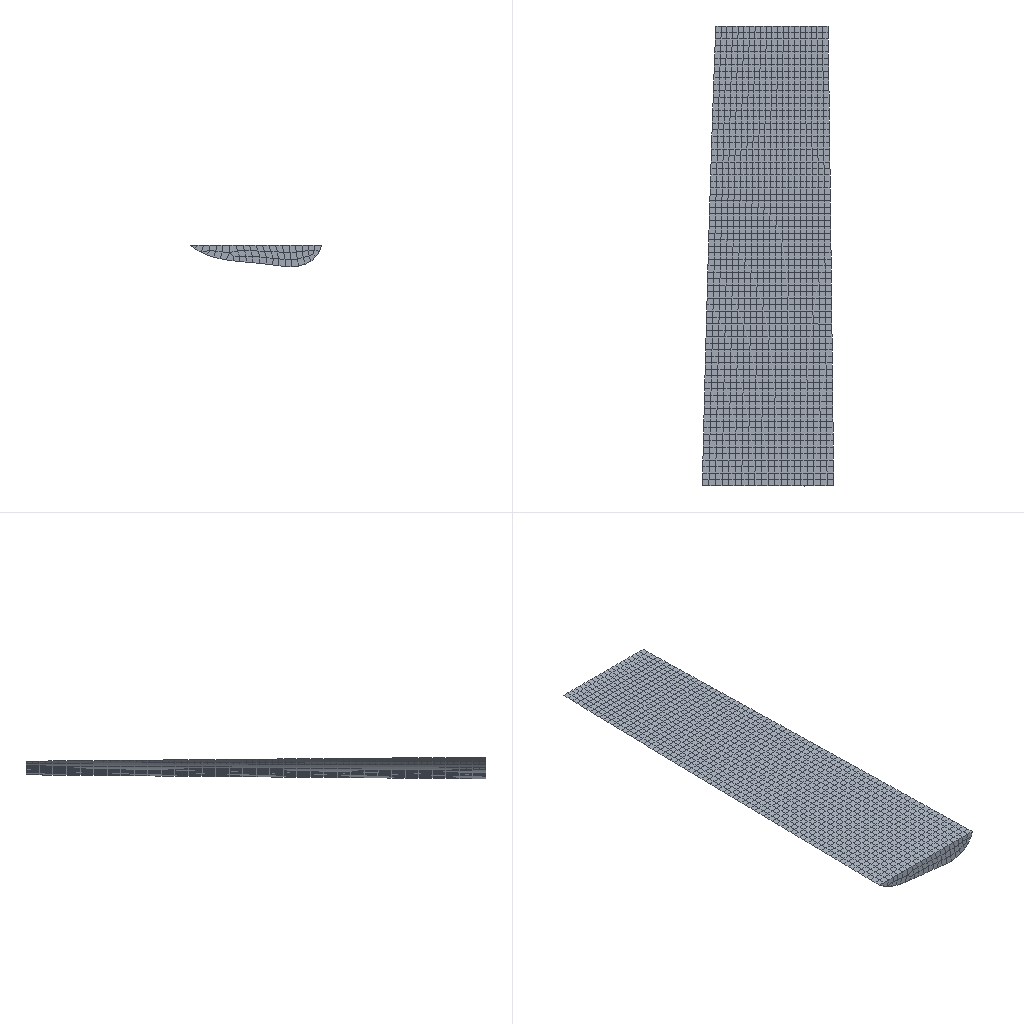Simulation study | ansys workbench
Ansys APDL input file, long lists of numbers shortened:
/batch
/config,noeldb,1     ! force off writing results to database
*get,_wallstrt,active,,time,wall
! ANSYS input file written by Workbench version 2022 R1
! File used for geometry attach:
/title,wbnew--____ (B5)
! ****** Begin Custom Load Command Snippet ******
/COM, ACT Extensions:
/COM,     LSDYNA, 2021.1
/COM,
! ****** End   Custom Load Command Snippet ******
*DIM,_wb_ProjectScratch_dir,string,248
_wb_ProjectScratch_dir(1) = ''
*DIM,_wb_SolverFiles_dir,string,248
_wb_SolverFiles_dir(1) = ''
*DIM,_wb_userfiles_dir,string,248
_wb_userfiles_dir(1) = ''
/com,--- Data in consistent NMM units. See Solving Units in the help system for more information.
/units,MPA
/nopr
/wb,file,start              !  signify a WB generated input file
/prep7
! Turn off shape checking because checks already performed inside WB mesher.
! See help system for more information.
SHPP,OFF,,NOWARN
/nolist
etcon,set             ! allow ANSYS to choose best KEYOP's for 180x elements, resets any applicable keyopt to MAPDL defaults
/com,*********** Nodes for the whole assembly ***********
nblock,3,,21303
(1i9,3e20.9e3)
        1     1.781042976E+01     6.901413409E+01    -1.589842969E+00
! (19366 more lines like these left out)
-1
/wb,elem,start            !  set before creation of elements
/com,*********** Elements for Body 1 "___7-FreeParts|__-__1" ***********
et,1,186
keyo,1,2,1          ! set full integration on SOLID186
eblock,19,solid,,3692
(19i9)
        1        1        1        1        0        0        0        0       20        0        1        1       16       17       31     2201     2186     2185     2171
! (7383 more lines like these left out)
-1
/wb,elem,end               !  done creating elements
/com,*********** Send User Defined Coordinate System(s) ***********
csys,0
toffst,273.15,  ! Temperature offset from absolute zero
/com,*********** Set Reference Temperature ***********
tref,22.
/wb,mat,start              !  starting to send materials
/com,*********** Send Materials ***********
Temperature = 'TEMP' ! Temperature
MP,DENS,1,7.85e-09,	! tonne mm^-3
MP,ALPX,1,1.2e-05,	! C^-1
MP,C,1,434000000,	! mm^2 s^-2 C^-1
MP,KXX,1,60.5,	! tonne mm s^-3 C^-1
MP,RSVX,1,0.00017,	! ohm mm
MP,EX,1,200000,	! tonne s^-2 mm^-1
MP,NUXY,1,0.3,
MP,MURX,1,10000,
/wb,mat,end                !  done sending materials
!************************* Model Summary ********************
!___7-FreeParts|__-__1,	结构钢,	matid,	1
!************************* End Model Summary ********************
! get the diagonal of the bounding box. Needed later for other things
*get,_xmin,node,,mnloc,x
*get,_ymin,node,,mnloc,y
*get,_zmin,node,,mnloc,z
*get,_xmax,node,,mxloc,x
*get,_ymax,node,,mxloc,y
*get,_zmax,node,,mxloc,z
_ASMDIAG=(_xmax-_xmin)*(_xmax-_xmin)+(_ymax-_ymin)*(_ymax-_ymin)+(_zmax-_zmin)*(_zmax-_zmin)
_ASMDIAG=SQRT(_ASMDIAG)
/wb,contact,start          !  starting to send contact
/wb,contact,end            !  done creating contacts
/golist
/wb,load,start             !  starting to send loads
/com,*********** Fixed Supports ***********
CMBLOCK,_FIXEDSU,NODE,      197
(8i10)
      2202      2203      2204      2205      2206      2207      2208      2209
! (24 more lines like these left out)
cmsel,s,_FIXEDSU
d,all,all
nsel,all
/com,*********** Define Force Using Surface Effect Elements ***********
local,12,0,0.,0.,0.,0.,0.,0.
csys,0
et,2,154
eblock,10,,,1562
(15i9)
     6779        2        2        2       12     3837     2275     2253     2252    13306    13262    13259    13260
! (1561 more lines like these left out)
-1
esel,s,type,,2
keyop,2,2,1                ! Apply load in local coordinate system
keyop,2,7,1                ! Use original area so load is constant in large deformation
esel,all
/gst,on,on
fini
*get,_numnode,node,0,count
*get,_numelem,elem,0,count
*get, _MAXELEMNUM, elem, 0, NUM, MAX
*get, _MAXNODENUM, node, 0, NUM, MAX
*get, _MAXELEMTYPE, etyp, 0, NUM, MAX
*get, _MAXREALCONST, real, 0, NUM, MAX
/go
/wb,load,end               !  done creating loads
/com,--- Number of total nodes = %_numnode%
/com,--- Number of contact elements = 1562
/com,--- Number of spring elements = 0
/com,--- Number of bearing elements = 0
/com,--- Number of solid elements = 3692
/com,--- Number of condensed parts = 0
/com,--- Number of total elements = %_numelem%
*get,_wallbsol,active,,time,wall
/com,****************************************************************************
/com,*************************    SOLUTION       ********************************
/com,****************************************************************************
/solu
antype,0                   ! static analysis
_thickRatio=  1     ! Ratio of thick parts in the model
eqsl,pcg,1e-8,,,,,,1
cntr,print,1               ! print out contact info and also make no initial contact an error
dmpoption,emat,no             ! Don't combine emat file for DANSYS
dmpoption,esav,no             ! Don't combine esav file for DANSYS
nldiag,cont,iter           ! print out contact info each equilibrium iteration
rescontrol,,none                 ! Do not keep any restart files
/com,****************************************************
/com,******************* SOLVE FOR LS 1 OF 1 ****************
esel,s,type,,2
nsle
sfe,all,1,pres,1,-204.694
sfe,all,2,pres,1,0.
sfe,all,3,pres,1,0.
nsel,all
esel,all
/nopr
/gopr
nsub,1,1,1
time,1.
outres,erase
outres,all,none
outres,nsol,all,
outres,rsol,all
outres,eangl,all
outres,etmp,all
outres,veng,all
outres,strs,all,
outres,epel,all,
outres,eppl,all,
outres,cont,all,
! *********** WB SOLVE COMMAND ***********
! check interactive state
*get,ANSINTER_,active,,int
*if,ANSINTER_,ne,0,then
/eof
*endif
solve
/com *************** Write FE CONNECTORS *********
CEWRITE,file,ce,,INTE
/com,****************************************************
/com,*************** FINISHED SOLVE FOR LS 1 *************
*get,_wallasol,active,,time,wall
/nopr
*get,_numnode,node,0,count
*get,_numelem,elem,0,count
*get, _MAXELEMNUM, elem, 0, NUM, MAX
*get, _MAXNODENUM, node, 0, NUM, MAX,,,INTERNAL
*get, _MAXELEMTYPE, etyp, 0, NUM, MAX
*get, _MAXREALCONST, real, 0, NUM, MAX
/gopr
*get,_PCGITER,active,,solu,cgiter
/post1
xmlo,ENCODING,ISO-8859-1
xmlo,parm
/xml,parm,xml
fini
/gopr
*get,_walldone,active,,time,wall
_preptime=(_wallbsol-_wallstrt)*3600
_solvtime=(_wallasol-_wallbsol)*3600
_posttime=(_walldone-_wallasol)*3600
_totaltim=(_walldone-_wallstrt)*3600
*get,_dlbratio,active,0,solu,dlbr
*get,_combtime,active,0,solu,comb
*get,_ssmode,active,0,solu,ssmm
*get,_ndofs,active,0,solu,ndof
*get,_sol_end_time,active,0,set,time
*if,_sol_end_time,eq,1.,then
/fclean				!clean distributed files
*endif
/com,--- Total number of nodes = %_numnode%
/com,--- Total number of elements = %_numelem%
/com,--- Element load balance ratio = %_dlbratio%
/com,--- Time to combine distributed files = %_combtime%
/com,--- Sparse memory mode = %_ssmode%
/com,--- Number of DOF = %_ndofs%
/wb,file,end               ! done with WB generated input